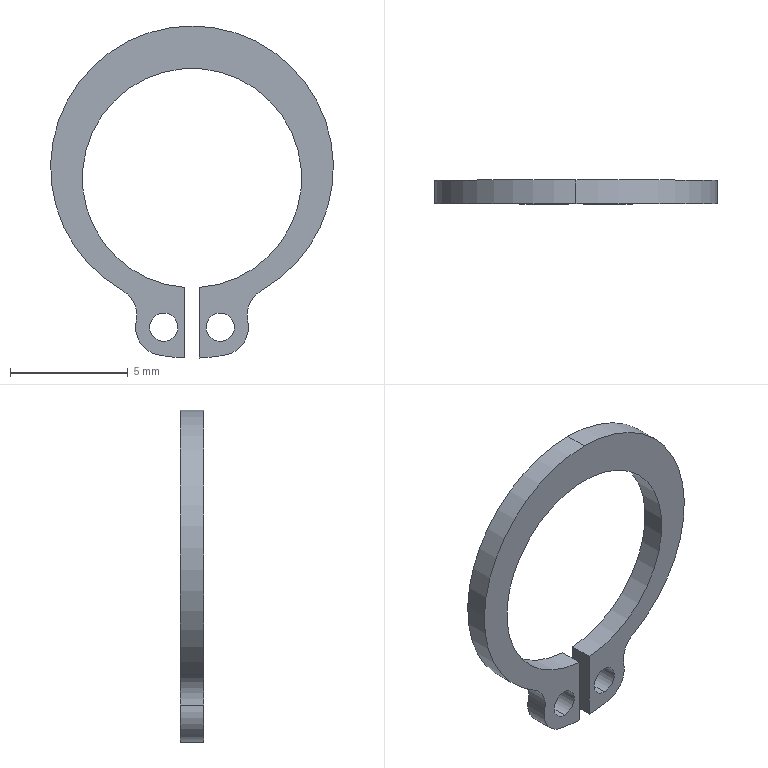Part | STEP file | C-type retaining ring STWS10_MISUMI_default | 1 solid | 17 faces | box 12 x 1 x 14.09 mm | volume 51.059 mm3 | cylinder 13 | plane 4 | commonest cylinder face diameters 1.2 x4 2.4 x4 12 x2 15.292 x2 9.3 x1
STEP:
#1=CARTESIAN_POINT('',(0.,-1.,6.45));
#2=VERTEX_POINT('',#1);
#3=CARTESIAN_POINT('',(-2.953,-1.,-4.773));
#4=VERTEX_POINT('',#3);
#5=CARTESIAN_POINT('',(0.,-1.,0.45));
#6=DIRECTION('',(0.,-1.,0.));
#7=DIRECTION('',(0.,0.,1.));
#8=AXIS2_PLACEMENT_3D('',#5,#6,#7);
#9=CIRCLE('',#8,6.);
#10=EDGE_CURVE('',#2,#4,#9,.T.);
#11=ORIENTED_EDGE('',*,*,#10,.F.);
#12=CARTESIAN_POINT('',(0.,0.,6.45));
#13=VERTEX_POINT('',#12);
#14=CARTESIAN_POINT('',(0.,-1.,6.45));
#15=DIRECTION('',(0.,1.,0.));
#16=VECTOR('',#15,1000.);
#17=LINE('',#14,#16);
#18=EDGE_CURVE('',#2,#13,#17,.T.);
#19=ORIENTED_EDGE('',*,*,#18,.T.);
#20=CARTESIAN_POINT('',(-2.953,0.,-4.773));
#21=VERTEX_POINT('',#20);
#22=CARTESIAN_POINT('',(0.,0.,0.45));
#23=DIRECTION('',(0.,-1.,0.));
#24=DIRECTION('',(0.,0.,1.));
#25=AXIS2_PLACEMENT_3D('',#22,#23,#24);
#26=CIRCLE('',#25,6.);
#27=EDGE_CURVE('',#13,#21,#26,.T.);
#28=ORIENTED_EDGE('',*,*,#27,.T.);
#29=CARTESIAN_POINT('',(-2.953,0.,-4.773));
#30=DIRECTION('',(0.,-1.,0.));
#31=VECTOR('',#30,1000.);
#32=LINE('',#29,#31);
#33=EDGE_CURVE('',#21,#4,#32,.T.);
#34=ORIENTED_EDGE('',*,*,#33,.T.);
#35=EDGE_LOOP('',(#11,#19,#28,#34));
#36=FACE_OUTER_BOUND('',#35,.T.);
#37=CARTESIAN_POINT('',(0.,-1.,0.45));
#38=DIRECTION('',(0.,1.,0.));
#39=DIRECTION('',(0.,0.,1.));
#40=AXIS2_PLACEMENT_3D('',#37,#38,#39);
#41=CYLINDRICAL_SURFACE('',#40,6.);
#42=ADVANCED_FACE('',(#36),#41,.T.);
#43=CARTESIAN_POINT('',(-1.2,0.,-5.734));
#44=VERTEX_POINT('',#43);
#45=CARTESIAN_POINT('',(-1.2,0.,-6.934));
#46=VERTEX_POINT('',#45);
#47=CARTESIAN_POINT('',(-1.2,0.,-6.334));
#48=DIRECTION('',(0.,-1.,0.));
#49=DIRECTION('',(0.,0.,-1.));
#50=AXIS2_PLACEMENT_3D('',#47,#48,#49);
#51=CIRCLE('',#50,0.6);
#52=EDGE_CURVE('',#44,#46,#51,.T.);
#53=ORIENTED_EDGE('',*,*,#52,.F.);
#54=CARTESIAN_POINT('',(-1.2,-1.,-5.734));
#55=VERTEX_POINT('',#54);
#56=CARTESIAN_POINT('',(-1.2,0.,-5.734));
#57=DIRECTION('',(0.,-1.,0.));
#58=VECTOR('',#57,1000.);
#59=LINE('',#56,#58);
#60=EDGE_CURVE('',#44,#55,#59,.T.);
#61=ORIENTED_EDGE('',*,*,#60,.T.);
#62=CARTESIAN_POINT('',(-1.2,-1.,-6.934));
#63=VERTEX_POINT('',#62);
#64=CARTESIAN_POINT('',(-1.2,-1.,-6.334));
#65=DIRECTION('',(0.,1.,0.));
#66=DIRECTION('',(0.,0.,-1.));
#67=AXIS2_PLACEMENT_3D('',#64,#65,#66);
#68=CIRCLE('',#67,0.6);
#69=EDGE_CURVE('',#63,#55,#68,.T.);
#70=ORIENTED_EDGE('',*,*,#69,.F.);
#71=CARTESIAN_POINT('',(-1.2,0.,-6.934));
#72=DIRECTION('',(0.,-1.,0.));
#73=VECTOR('',#72,1000.);
#74=LINE('',#71,#73);
#75=EDGE_CURVE('',#46,#63,#74,.T.);
#76=ORIENTED_EDGE('',*,*,#75,.F.);
#77=EDGE_LOOP('',(#53,#61,#70,#76));
#78=FACE_OUTER_BOUND('',#77,.T.);
#79=CARTESIAN_POINT('',(-1.2,0.,-6.334));
#80=DIRECTION('',(0.,-1.,0.));
#81=DIRECTION('',(0.,0.,-1.));
#82=AXIS2_PLACEMENT_3D('',#79,#80,#81);
#83=CYLINDRICAL_SURFACE('',#82,0.6);
#84=ADVANCED_FACE('',(#78),#83,.F.);
#85=CARTESIAN_POINT('',(1.2,0.,-5.734));
#86=VERTEX_POINT('',#85);
#87=CARTESIAN_POINT('',(1.2,0.,-6.934));
#88=VERTEX_POINT('',#87);
#89=CARTESIAN_POINT('',(1.2,0.,-6.334));
#90=DIRECTION('',(0.,-1.,0.));
#91=DIRECTION('',(0.,0.,-1.));
#92=AXIS2_PLACEMENT_3D('',#89,#90,#91);
#93=CIRCLE('',#92,0.6);
#94=EDGE_CURVE('',#86,#88,#93,.T.);
#95=ORIENTED_EDGE('',*,*,#94,.F.);
#96=CARTESIAN_POINT('',(1.2,-1.,-5.734));
#97=VERTEX_POINT('',#96);
#98=CARTESIAN_POINT('',(1.2,0.,-5.734));
#99=DIRECTION('',(0.,-1.,0.));
#100=VECTOR('',#99,1000.);
#101=LINE('',#98,#100);
#102=EDGE_CURVE('',#86,#97,#101,.T.);
#103=ORIENTED_EDGE('',*,*,#102,.T.);
#104=CARTESIAN_POINT('',(1.2,-1.,-6.934));
#105=VERTEX_POINT('',#104);
#106=CARTESIAN_POINT('',(1.2,-1.,-6.334));
#107=DIRECTION('',(0.,1.,0.));
#108=DIRECTION('',(0.,0.,-1.));
#109=AXIS2_PLACEMENT_3D('',#106,#107,#108);
#110=CIRCLE('',#109,0.6);
#111=EDGE_CURVE('',#105,#97,#110,.T.);
#112=ORIENTED_EDGE('',*,*,#111,.F.);
#113=CARTESIAN_POINT('',(1.2,0.,-6.934));
#114=DIRECTION('',(0.,-1.,0.));
#115=VECTOR('',#114,1000.);
#116=LINE('',#113,#115);
#117=EDGE_CURVE('',#88,#105,#116,.T.);
#118=ORIENTED_EDGE('',*,*,#117,.F.);
#119=EDGE_LOOP('',(#95,#103,#112,#118));
#120=FACE_OUTER_BOUND('',#119,.T.);
#121=CARTESIAN_POINT('',(1.2,0.,-6.334));
#122=DIRECTION('',(0.,-1.,0.));
#123=DIRECTION('',(0.,0.,-1.));
#124=AXIS2_PLACEMENT_3D('',#121,#122,#123);
#125=CYLINDRICAL_SURFACE('',#124,0.6);
#126=ADVANCED_FACE('',(#120),#125,.F.);
#127=CARTESIAN_POINT('',(2.953,-1.,-4.773));
#128=VERTEX_POINT('',#127);
#129=CARTESIAN_POINT('',(0.,-1.,0.45));
#130=DIRECTION('',(0.,-1.,0.));
#131=DIRECTION('',(0.,0.,1.));
#132=AXIS2_PLACEMENT_3D('',#129,#130,#131);
#133=CIRCLE('',#132,6.);
#134=EDGE_CURVE('',#128,#2,#133,.T.);
#135=ORIENTED_EDGE('',*,*,#134,.T.);
#136=ORIENTED_EDGE('',*,*,#10,.T.);
#137=CARTESIAN_POINT('',(-2.372,-1.,-6.075));
#138=VERTEX_POINT('',#137);
#139=CARTESIAN_POINT('',(-3.544,-1.,-5.817));
#140=DIRECTION('',(0.,1.,0.));
#141=DIRECTION('',(0.,0.,-1.));
#142=AXIS2_PLACEMENT_3D('',#139,#140,#141);
#143=CIRCLE('',#142,1.2);
#144=EDGE_CURVE('',#4,#138,#143,.T.);
#145=ORIENTED_EDGE('',*,*,#144,.T.);
#146=CARTESIAN_POINT('',(-1.423,-1.,-7.513));
#147=VERTEX_POINT('',#146);
#148=CARTESIAN_POINT('',(-1.2,-1.,-6.334));
#149=DIRECTION('',(0.,-1.,0.));
#150=DIRECTION('',(0.,0.,1.));
#151=AXIS2_PLACEMENT_3D('',#148,#149,#150);
#152=CIRCLE('',#151,1.2);
#153=EDGE_CURVE('',#138,#147,#152,.T.);
#154=ORIENTED_EDGE('',*,*,#153,.T.);
#155=CARTESIAN_POINT('',(-0.3,-1.,-7.64));
#156=VERTEX_POINT('',#155);
#157=CARTESIAN_POINT('',(0.,-1.,0.));
#158=DIRECTION('',(0.,-1.,0.));
#159=DIRECTION('',(0.,0.,1.));
#160=AXIS2_PLACEMENT_3D('',#157,#158,#159);
#161=CIRCLE('',#160,7.646);
#162=EDGE_CURVE('',#147,#156,#161,.T.);
#163=ORIENTED_EDGE('',*,*,#162,.T.);
#164=CARTESIAN_POINT('',(-0.3,-1.,-4.64));
#165=VERTEX_POINT('',#164);
#166=CARTESIAN_POINT('',(-0.3,-1.,-7.64));
#167=DIRECTION('',(0.,0.,1.));
#168=VECTOR('',#167,1000.);
#169=LINE('',#166,#168);
#170=EDGE_CURVE('',#156,#165,#169,.T.);
#171=ORIENTED_EDGE('',*,*,#170,.T.);
#172=CARTESIAN_POINT('',(0.3,-1.,-4.64));
#173=VERTEX_POINT('',#172);
#174=CARTESIAN_POINT('',(0.,-1.,0.));
#175=DIRECTION('',(0.,1.,0.));
#176=DIRECTION('',(0.,0.,-1.));
#177=AXIS2_PLACEMENT_3D('',#174,#175,#176);
#178=CIRCLE('',#177,4.65);
#179=EDGE_CURVE('',#165,#173,#178,.T.);
#180=ORIENTED_EDGE('',*,*,#179,.T.);
#181=CARTESIAN_POINT('',(0.3,-1.,-7.64));
#182=VERTEX_POINT('',#181);
#183=CARTESIAN_POINT('',(0.3,-1.,-7.64));
#184=DIRECTION('',(0.,0.,-1.));
#185=VECTOR('',#184,1000.);
#186=LINE('',#183,#185);
#187=EDGE_CURVE('',#173,#182,#186,.T.);
#188=ORIENTED_EDGE('',*,*,#187,.T.);
#189=CARTESIAN_POINT('',(1.423,-1.,-7.513));
#190=VERTEX_POINT('',#189);
#191=CARTESIAN_POINT('',(0.,-1.,0.));
#192=DIRECTION('',(0.,-1.,0.));
#193=DIRECTION('',(0.,0.,1.));
#194=AXIS2_PLACEMENT_3D('',#191,#192,#193);
#195=CIRCLE('',#194,7.646);
#196=EDGE_CURVE('',#182,#190,#195,.T.);
#197=ORIENTED_EDGE('',*,*,#196,.T.);
#198=CARTESIAN_POINT('',(2.372,-1.,-6.075));
#199=VERTEX_POINT('',#198);
#200=CARTESIAN_POINT('',(1.2,-1.,-6.334));
#201=DIRECTION('',(0.,-1.,0.));
#202=DIRECTION('',(0.,0.,1.));
#203=AXIS2_PLACEMENT_3D('',#200,#201,#202);
#204=CIRCLE('',#203,1.2);
#205=EDGE_CURVE('',#190,#199,#204,.T.);
#206=ORIENTED_EDGE('',*,*,#205,.T.);
#207=CARTESIAN_POINT('',(3.544,-1.,-5.817));
#208=DIRECTION('',(0.,1.,0.));
#209=DIRECTION('',(0.,0.,-1.));
#210=AXIS2_PLACEMENT_3D('',#207,#208,#209);
#211=CIRCLE('',#210,1.2);
#212=EDGE_CURVE('',#199,#128,#211,.T.);
#213=ORIENTED_EDGE('',*,*,#212,.T.);
#214=EDGE_LOOP('',(#135,#136,#145,#154,#163,#171,#180,#188,#197,#206,#213));
#215=FACE_OUTER_BOUND('',#214,.T.);
#216=ORIENTED_EDGE('',*,*,#69,.T.);
#217=CARTESIAN_POINT('',(-1.2,-1.,-6.334));
#218=DIRECTION('',(0.,1.,0.));
#219=DIRECTION('',(0.,0.,-1.));
#220=AXIS2_PLACEMENT_3D('',#217,#218,#219);
#221=CIRCLE('',#220,0.6);
#222=EDGE_CURVE('',#55,#63,#221,.T.);
#223=ORIENTED_EDGE('',*,*,#222,.T.);
#224=EDGE_LOOP('',(#216,#223));
#225=FACE_BOUND('',#224,.T.);
#226=ORIENTED_EDGE('',*,*,#111,.T.);
#227=CARTESIAN_POINT('',(1.2,-1.,-6.334));
#228=DIRECTION('',(0.,1.,0.));
#229=DIRECTION('',(0.,0.,-1.));
#230=AXIS2_PLACEMENT_3D('',#227,#228,#229);
#231=CIRCLE('',#230,0.6);
#232=EDGE_CURVE('',#97,#105,#231,.T.);
#233=ORIENTED_EDGE('',*,*,#232,.T.);
#234=EDGE_LOOP('',(#226,#233));
#235=FACE_BOUND('',#234,.T.);
#236=CARTESIAN_POINT('',(-6.121,-1.,-7.64));
#237=DIRECTION('',(0.,-1.,0.));
#238=DIRECTION('',(0.,0.,-1.));
#239=AXIS2_PLACEMENT_3D('',#236,#237,#238);
#240=PLANE('',#239);
#241=ADVANCED_FACE('',(#215,#225,#235),#240,.T.);
#242=CARTESIAN_POINT('',(-2.372,0.,-6.075));
#243=VERTEX_POINT('',#242);
#244=CARTESIAN_POINT('',(-2.372,0.,-6.075));
#245=DIRECTION('',(0.,1.,0.));
#246=VECTOR('',#245,1000.);
#247=LINE('',#244,#246);
#248=EDGE_CURVE('',#138,#243,#247,.T.);
#249=ORIENTED_EDGE('',*,*,#248,.F.);
#250=ORIENTED_EDGE('',*,*,#144,.F.);
#251=ORIENTED_EDGE('',*,*,#33,.F.);
#252=CARTESIAN_POINT('',(-3.544,0.,-5.817));
#253=DIRECTION('',(0.,-1.,0.));
#254=DIRECTION('',(0.,0.,-1.));
#255=AXIS2_PLACEMENT_3D('',#252,#253,#254);
#256=CIRCLE('',#255,1.2);
#257=EDGE_CURVE('',#243,#21,#256,.T.);
#258=ORIENTED_EDGE('',*,*,#257,.F.);
#259=EDGE_LOOP('',(#249,#250,#251,#258));
#260=FACE_OUTER_BOUND('',#259,.T.);
#261=CARTESIAN_POINT('',(-3.544,0.,-5.817));
#262=DIRECTION('',(0.,-1.,0.));
#263=DIRECTION('',(0.,0.,-1.));
#264=AXIS2_PLACEMENT_3D('',#261,#262,#263);
#265=CYLINDRICAL_SURFACE('',#264,1.2);
#266=ADVANCED_FACE('',(#260),#265,.F.);
#267=ORIENTED_EDGE('',*,*,#18,.F.);
#268=ORIENTED_EDGE('',*,*,#134,.F.);
#269=CARTESIAN_POINT('',(2.953,0.,-4.773));
#270=VERTEX_POINT('',#269);
#271=CARTESIAN_POINT('',(2.953,-1.,-4.773));
#272=DIRECTION('',(0.,1.,0.));
#273=VECTOR('',#272,1000.);
#274=LINE('',#271,#273);
#275=EDGE_CURVE('',#128,#270,#274,.T.);
#276=ORIENTED_EDGE('',*,*,#275,.T.);
#277=CARTESIAN_POINT('',(0.,0.,0.45));
#278=DIRECTION('',(0.,-1.,0.));
#279=DIRECTION('',(0.,0.,1.));
#280=AXIS2_PLACEMENT_3D('',#277,#278,#279);
#281=CIRCLE('',#280,6.);
#282=EDGE_CURVE('',#270,#13,#281,.T.);
#283=ORIENTED_EDGE('',*,*,#282,.T.);
#284=EDGE_LOOP('',(#267,#268,#276,#283));
#285=FACE_OUTER_BOUND('',#284,.T.);
#286=CARTESIAN_POINT('',(0.,-1.,0.45));
#287=DIRECTION('',(0.,1.,0.));
#288=DIRECTION('',(0.,0.,1.));
#289=AXIS2_PLACEMENT_3D('',#286,#287,#288);
#290=CYLINDRICAL_SURFACE('',#289,6.);
#291=ADVANCED_FACE('',(#285),#290,.T.);
#292=ORIENTED_EDGE('',*,*,#275,.F.);
#293=ORIENTED_EDGE('',*,*,#212,.F.);
#294=CARTESIAN_POINT('',(2.372,0.,-6.075));
#295=VERTEX_POINT('',#294);
#296=CARTESIAN_POINT('',(2.372,0.,-6.075));
#297=DIRECTION('',(0.,-1.,0.));
#298=VECTOR('',#297,1000.);
#299=LINE('',#296,#298);
#300=EDGE_CURVE('',#295,#199,#299,.T.);
#301=ORIENTED_EDGE('',*,*,#300,.F.);
#302=CARTESIAN_POINT('',(3.544,0.,-5.817));
#303=DIRECTION('',(0.,-1.,0.));
#304=DIRECTION('',(0.,0.,-1.));
#305=AXIS2_PLACEMENT_3D('',#302,#303,#304);
#306=CIRCLE('',#305,1.2);
#307=EDGE_CURVE('',#270,#295,#306,.T.);
#308=ORIENTED_EDGE('',*,*,#307,.F.);
#309=EDGE_LOOP('',(#292,#293,#301,#308));
#310=FACE_OUTER_BOUND('',#309,.T.);
#311=CARTESIAN_POINT('',(3.544,0.,-5.817));
#312=DIRECTION('',(0.,-1.,0.));
#313=DIRECTION('',(0.,0.,-1.));
#314=AXIS2_PLACEMENT_3D('',#311,#312,#313);
#315=CYLINDRICAL_SURFACE('',#314,1.2);
#316=ADVANCED_FACE('',(#310),#315,.F.);
#317=ORIENTED_EDGE('',*,*,#205,.F.);
#318=CARTESIAN_POINT('',(1.423,0.,-7.513));
#319=VERTEX_POINT('',#318);
#320=CARTESIAN_POINT('',(1.423,-1.,-7.513));
#321=DIRECTION('',(0.,1.,0.));
#322=VECTOR('',#321,1000.);
#323=LINE('',#320,#322);
#324=EDGE_CURVE('',#190,#319,#323,.T.);
#325=ORIENTED_EDGE('',*,*,#324,.T.);
#326=CARTESIAN_POINT('',(1.2,0.,-6.334));
#327=DIRECTION('',(0.,-1.,0.));
#328=DIRECTION('',(0.,0.,1.));
#329=AXIS2_PLACEMENT_3D('',#326,#327,#328);
#330=CIRCLE('',#329,1.2);
#331=EDGE_CURVE('',#319,#295,#330,.T.);
#332=ORIENTED_EDGE('',*,*,#331,.T.);
#333=ORIENTED_EDGE('',*,*,#300,.T.);
#334=EDGE_LOOP('',(#317,#325,#332,#333));
#335=FACE_OUTER_BOUND('',#334,.T.);
#336=CARTESIAN_POINT('',(1.2,-1.,-6.334));
#337=DIRECTION('',(0.,1.,0.));
#338=DIRECTION('',(0.,0.,1.));
#339=AXIS2_PLACEMENT_3D('',#336,#337,#338);
#340=CYLINDRICAL_SURFACE('',#339,1.2);
#341=ADVANCED_FACE('',(#335),#340,.T.);
#342=ORIENTED_EDGE('',*,*,#196,.F.);
#343=CARTESIAN_POINT('',(0.3,0.,-7.64));
#344=VERTEX_POINT('',#343);
#345=CARTESIAN_POINT('',(0.3,-1.,-7.64));
#346=DIRECTION('',(0.,1.,0.));
#347=VECTOR('',#346,1000.);
#348=LINE('',#345,#347);
#349=EDGE_CURVE('',#182,#344,#348,.T.);
#350=ORIENTED_EDGE('',*,*,#349,.T.);
#351=CARTESIAN_POINT('',(0.,0.,0.));
#352=DIRECTION('',(0.,-1.,0.));
#353=DIRECTION('',(0.,0.,1.));
#354=AXIS2_PLACEMENT_3D('',#351,#352,#353);
#355=CIRCLE('',#354,7.646);
#356=EDGE_CURVE('',#344,#319,#355,.T.);
#357=ORIENTED_EDGE('',*,*,#356,.T.);
#358=ORIENTED_EDGE('',*,*,#324,.F.);
#359=EDGE_LOOP('',(#342,#350,#357,#358));
#360=FACE_OUTER_BOUND('',#359,.T.);
#361=CARTESIAN_POINT('',(0.,-1.,0.));
#362=DIRECTION('',(0.,1.,0.));
#363=DIRECTION('',(0.,0.,1.));
#364=AXIS2_PLACEMENT_3D('',#361,#362,#363);
#365=CYLINDRICAL_SURFACE('',#364,7.646);
#366=ADVANCED_FACE('',(#360),#365,.T.);
#367=CARTESIAN_POINT('',(0.3,0.,-4.64));
#368=VERTEX_POINT('',#367);
#369=CARTESIAN_POINT('',(0.3,0.,-4.64));
#370=DIRECTION('',(0.,1.,0.));
#371=VECTOR('',#370,1000.);
#372=LINE('',#369,#371);
#373=EDGE_CURVE('',#173,#368,#372,.T.);
#374=ORIENTED_EDGE('',*,*,#373,.T.);
#375=CARTESIAN_POINT('',(0.3,0.,-7.64));
#376=DIRECTION('',(0.,0.,-1.));
#377=VECTOR('',#376,1000.);
#378=LINE('',#375,#377);
#379=EDGE_CURVE('',#368,#344,#378,.T.);
#380=ORIENTED_EDGE('',*,*,#379,.T.);
#381=ORIENTED_EDGE('',*,*,#349,.F.);
#382=ORIENTED_EDGE('',*,*,#187,.F.);
#383=EDGE_LOOP('',(#374,#380,#381,#382));
#384=FACE_OUTER_BOUND('',#383,.T.);
#385=CARTESIAN_POINT('',(0.3,0.,-7.64));
#386=DIRECTION('',(-1.,0.,0.));
#387=DIRECTION('',(0.,0.,1.));
#388=AXIS2_PLACEMENT_3D('',#385,#386,#387);
#389=PLANE('',#388);
#390=ADVANCED_FACE('',(#384),#389,.T.);
#391=CARTESIAN_POINT('',(-0.3,0.,-4.64));
#392=VERTEX_POINT('',#391);
#393=CARTESIAN_POINT('',(0.,0.,0.));
#394=DIRECTION('',(0.,-1.,0.));
#395=DIRECTION('',(0.,0.,-1.));
#396=AXIS2_PLACEMENT_3D('',#393,#394,#395);
#397=CIRCLE('',#396,4.65);
#398=EDGE_CURVE('',#368,#392,#397,.T.);
#399=ORIENTED_EDGE('',*,*,#398,.F.);
#400=ORIENTED_EDGE('',*,*,#373,.F.);
#401=ORIENTED_EDGE('',*,*,#179,.F.);
#402=CARTESIAN_POINT('',(-0.3,0.,-4.64));
#403=DIRECTION('',(0.,-1.,0.));
#404=VECTOR('',#403,1000.);
#405=LINE('',#402,#404);
#406=EDGE_CURVE('',#392,#165,#405,.T.);
#407=ORIENTED_EDGE('',*,*,#406,.F.);
#408=EDGE_LOOP('',(#399,#400,#401,#407));
#409=FACE_OUTER_BOUND('',#408,.T.);
#410=CARTESIAN_POINT('',(0.,0.,0.));
#411=DIRECTION('',(0.,-1.,0.));
#412=DIRECTION('',(0.,0.,-1.));
#413=AXIS2_PLACEMENT_3D('',#410,#411,#412);
#414=CYLINDRICAL_SURFACE('',#413,4.65);
#415=ADVANCED_FACE('',(#409),#414,.F.);
#416=ORIENTED_EDGE('',*,*,#406,.T.);
#417=ORIENTED_EDGE('',*,*,#170,.F.);
#418=CARTESIAN_POINT('',(-0.3,0.,-7.64));
#419=VERTEX_POINT('',#418);
#420=CARTESIAN_POINT('',(-0.3,-1.,-7.64));
#421=DIRECTION('',(0.,1.,0.));
#422=VECTOR('',#421,1000.);
#423=LINE('',#420,#422);
#424=EDGE_CURVE('',#156,#419,#423,.T.);
#425=ORIENTED_EDGE('',*,*,#424,.T.);
#426=CARTESIAN_POINT('',(-0.3,0.,-7.64));
#427=DIRECTION('',(0.,0.,1.));
#428=VECTOR('',#427,1000.);
#429=LINE('',#426,#428);
#430=EDGE_CURVE('',#419,#392,#429,.T.);
#431=ORIENTED_EDGE('',*,*,#430,.T.);
#432=EDGE_LOOP('',(#416,#417,#425,#431));
#433=FACE_OUTER_BOUND('',#432,.T.);
#434=CARTESIAN_POINT('',(-0.3,-1.,-7.64));
#435=DIRECTION('',(1.,0.,0.));
#436=DIRECTION('',(0.,0.,-1.));
#437=AXIS2_PLACEMENT_3D('',#434,#435,#436);
#438=PLANE('',#437);
#439=ADVANCED_FACE('',(#433),#438,.T.);
#440=ORIENTED_EDGE('',*,*,#162,.F.);
#441=CARTESIAN_POINT('',(-1.423,0.,-7.513));
#442=VERTEX_POINT('',#441);
#443=CARTESIAN_POINT('',(-1.423,-1.,-7.513));
#444=DIRECTION('',(0.,1.,0.));
#445=VECTOR('',#444,1000.);
#446=LINE('',#443,#445);
#447=EDGE_CURVE('',#147,#442,#446,.T.);
#448=ORIENTED_EDGE('',*,*,#447,.T.);
#449=CARTESIAN_POINT('',(0.,0.,0.));
#450=DIRECTION('',(0.,-1.,0.));
#451=DIRECTION('',(0.,0.,1.));
#452=AXIS2_PLACEMENT_3D('',#449,#450,#451);
#453=CIRCLE('',#452,7.646);
#454=EDGE_CURVE('',#442,#419,#453,.T.);
#455=ORIENTED_EDGE('',*,*,#454,.T.);
#456=ORIENTED_EDGE('',*,*,#424,.F.);
#457=EDGE_LOOP('',(#440,#448,#455,#456));
#458=FACE_OUTER_BOUND('',#457,.T.);
#459=CARTESIAN_POINT('',(0.,-1.,0.));
#460=DIRECTION('',(0.,1.,0.));
#461=DIRECTION('',(0.,0.,1.));
#462=AXIS2_PLACEMENT_3D('',#459,#460,#461);
#463=CYLINDRICAL_SURFACE('',#462,7.646);
#464=ADVANCED_FACE('',(#458),#463,.T.);
#465=ORIENTED_EDGE('',*,*,#153,.F.);
#466=ORIENTED_EDGE('',*,*,#248,.T.);
#467=CARTESIAN_POINT('',(-1.2,0.,-6.334));
#468=DIRECTION('',(0.,-1.,0.));
#469=DIRECTION('',(0.,0.,1.));
#470=AXIS2_PLACEMENT_3D('',#467,#468,#469);
#471=CIRCLE('',#470,1.2);
#472=EDGE_CURVE('',#243,#442,#471,.T.);
#473=ORIENTED_EDGE('',*,*,#472,.T.);
#474=ORIENTED_EDGE('',*,*,#447,.F.);
#475=EDGE_LOOP('',(#465,#466,#473,#474));
#476=FACE_OUTER_BOUND('',#475,.T.);
#477=CARTESIAN_POINT('',(-1.2,-1.,-6.334));
#478=DIRECTION('',(0.,1.,0.));
#479=DIRECTION('',(0.,0.,1.));
#480=AXIS2_PLACEMENT_3D('',#477,#478,#479);
#481=CYLINDRICAL_SURFACE('',#480,1.2);
#482=ADVANCED_FACE('',(#476),#481,.T.);
#483=ORIENTED_EDGE('',*,*,#60,.F.);
#484=CARTESIAN_POINT('',(-1.2,0.,-6.334));
#485=DIRECTION('',(0.,-1.,0.));
#486=DIRECTION('',(0.,0.,-1.));
#487=AXIS2_PLACEMENT_3D('',#484,#485,#486);
#488=CIRCLE('',#487,0.6);
#489=EDGE_CURVE('',#46,#44,#488,.T.);
#490=ORIENTED_EDGE('',*,*,#489,.F.);
#491=ORIENTED_EDGE('',*,*,#75,.T.);
#492=ORIENTED_EDGE('',*,*,#222,.F.);
#493=EDGE_LOOP('',(#483,#490,#491,#492));
#494=FACE_OUTER_BOUND('',#493,.T.);
#495=CARTESIAN_POINT('',(-1.2,0.,-6.334));
#496=DIRECTION('',(0.,-1.,0.));
#497=DIRECTION('',(0.,0.,-1.));
#498=AXIS2_PLACEMENT_3D('',#495,#496,#497);
#499=CYLINDRICAL_SURFACE('',#498,0.6);
#500=ADVANCED_FACE('',(#494),#499,.F.);
#501=ORIENTED_EDGE('',*,*,#102,.F.);
#502=CARTESIAN_POINT('',(1.2,0.,-6.334));
#503=DIRECTION('',(0.,-1.,0.));
#504=DIRECTION('',(0.,0.,-1.));
#505=AXIS2_PLACEMENT_3D('',#502,#503,#504);
#506=CIRCLE('',#505,0.6);
#507=EDGE_CURVE('',#88,#86,#506,.T.);
#508=ORIENTED_EDGE('',*,*,#507,.F.);
#509=ORIENTED_EDGE('',*,*,#117,.T.);
#510=ORIENTED_EDGE('',*,*,#232,.F.);
#511=EDGE_LOOP('',(#501,#508,#509,#510));
#512=FACE_OUTER_BOUND('',#511,.T.);
#513=CARTESIAN_POINT('',(1.2,0.,-6.334));
#514=DIRECTION('',(0.,-1.,0.));
#515=DIRECTION('',(0.,0.,-1.));
#516=AXIS2_PLACEMENT_3D('',#513,#514,#515);
#517=CYLINDRICAL_SURFACE('',#516,0.6);
#518=ADVANCED_FACE('',(#512),#517,.F.);
#519=ORIENTED_EDGE('',*,*,#331,.F.);
#520=ORIENTED_EDGE('',*,*,#356,.F.);
#521=ORIENTED_EDGE('',*,*,#379,.F.);
#522=ORIENTED_EDGE('',*,*,#398,.T.);
#523=ORIENTED_EDGE('',*,*,#430,.F.);
#524=ORIENTED_EDGE('',*,*,#454,.F.);
#525=ORIENTED_EDGE('',*,*,#472,.F.);
#526=ORIENTED_EDGE('',*,*,#257,.T.);
#527=ORIENTED_EDGE('',*,*,#27,.F.);
#528=ORIENTED_EDGE('',*,*,#282,.F.);
#529=ORIENTED_EDGE('',*,*,#307,.T.);
#530=EDGE_LOOP('',(#519,#520,#521,#522,#523,#524,#525,#526,#527,#528,#529));
#531=FACE_OUTER_BOUND('',#530,.T.);
#532=ORIENTED_EDGE('',*,*,#489,.T.);
#533=ORIENTED_EDGE('',*,*,#52,.T.);
#534=EDGE_LOOP('',(#532,#533));
#535=FACE_BOUND('',#534,.T.);
#536=ORIENTED_EDGE('',*,*,#507,.T.);
#537=ORIENTED_EDGE('',*,*,#94,.T.);
#538=EDGE_LOOP('',(#536,#537));
#539=FACE_BOUND('',#538,.T.);
#540=CARTESIAN_POINT('',(6.121,0.,-7.64));
#541=DIRECTION('',(0.,1.,0.));
#542=DIRECTION('',(0.,0.,1.));
#543=AXIS2_PLACEMENT_3D('',#540,#541,#542);
#544=PLANE('',#543);
#545=ADVANCED_FACE('',(#531,#535,#539),#544,.T.);
#546=CLOSED_SHELL('',(#42,#84,#126,#241,#266,#291,#316,#341,#366,#390,#415,#439,#464,#482,#500,#518,#545));
#547=MANIFOLD_SOLID_BREP('',#546);
#548=CARTESIAN_POINT('',(0.,0.,0.));
#549=DIRECTION('',(0.,0.,1.));
#550=DIRECTION('',(1.,0.,0.));
#551=AXIS2_PLACEMENT_3D('',#548,#549,#550);
#552=(LENGTH_UNIT()NAMED_UNIT(*)SI_UNIT(.MILLI.,.METRE.));
#553=UNCERTAINTY_MEASURE_WITH_UNIT(LENGTH_MEASURE(0.00001),#552,'','');
#554=(NAMED_UNIT(*)PLANE_ANGLE_UNIT()SI_UNIT($,.RADIAN.));
#555=(NAMED_UNIT(*)SI_UNIT($,.STERADIAN.)SOLID_ANGLE_UNIT());
#556=(GEOMETRIC_REPRESENTATION_CONTEXT(3)GLOBAL_UNCERTAINTY_ASSIGNED_CONTEXT((#553))GLOBAL_UNIT_ASSIGNED_CONTEXT((#552,#554,#555))REPRESENTATION_CONTEXT('',''));
#557=ADVANCED_BREP_SHAPE_REPRESENTATION('',(#547,#551),#556);